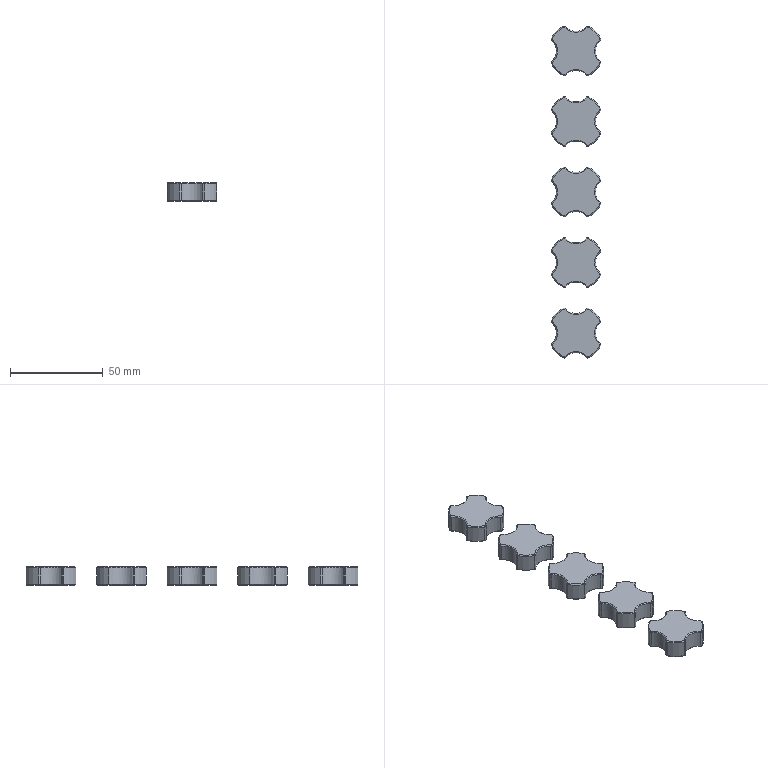NC program | NX | posted with a generic post | part box 26.875 x 178.875 x 10 mm
Whole program:
N10 G17 G21 G94 G90
(FLOOR_WALL_COPY , TOOL : D80)
N12 T19 M6
N14 G54
N16 G17 G0 G90 X-134.438 Y0. S6500 M3
N18 G43 Z30. H19
N20 Z7.5
N22 G94 G1 Z4.5 F1500.
N24 X-129.438
N26 X129.437
N28 X134.437
N30 Z7.5
N32 G0 Z30.
N34 X-134.438
N36 Z7.
N38 G1 Z4.
N40 X-129.438
N42 X129.437
N44 X134.437
N46 Z7.
N48 G0 Z30.
N50 X-134.438
N52 Z6.5
N54 G1 Z3.5
N56 X-129.438
N58 X129.437
N60 X134.437
N62 Z6.5
N64 G0 Z30.
N66 X-134.438
N68 Z6.
N70 G1 Z3.
N72 X-129.438
N74 X129.437
N76 X134.437
N78 Z6.
N80 G0 Z30.
N82 X-134.438
N84 Z5.5
N86 G1 Z2.5
N88 X-129.438
N90 X129.437
N92 X134.437
N94 Z5.5
N96 G0 Z30.
N98 X-134.438
N100 Z5.
N102 G1 Z2.
N104 X-129.438
N106 X129.437
N108 X134.437
N110 Z5.
N112 G0 Z30.
N114 X-134.438
N116 Z4.5
N118 G1 Z1.5
N120 X-129.438
N122 X129.437
N124 X134.437
N126 Z4.5
N128 G0 Z30.
N130 X-134.438
N132 Z4.
N134 G1 Z1.
N136 X-129.438
N138 X129.437
N140 X134.437
N142 Z4.
N144 G0 Z30.
N146 X-134.438
N148 Z3.5
N150 G1 Z0.5
N152 X-129.438
N154 X129.437
N156 X134.437
N158 Z3.5
N160 G0 Z30.
N162 X-134.438
N164 Z3.
N166 G1 Z0.
N168 X-129.438
N170 X129.437
N172 X134.437
N174 Z3.
N176 G0 Z30.
N178 M5
(PLANAR_MILL_COPY_COPY_COPY_COPY_COPY , TOOL : D6A45)
N180 T01 M6
N182 G54
N184 G17 G0 G90 X-64.945 Y12.28 S9500 M3
N186 G43 Z30. H1
N188 Z0.
N190 G94 G1 Z-1.5 F1250.
N192 G3 X-64.686 Y11.314 R1.
N194 G2 X-61.786 Y7.345 R16.
N196 X-62.254 Y4.915 R2.
N198 G3 X-62.254 Y-4.915 R6.5
N200 G2 X-61.786 Y-7.345 R2.
N202 X-68.655 Y-14.214 R16.
N204 X-71.085 Y-13.746 R2.
N206 G3 X-80.915 Y-13.746 R6.5
N208 G2 X-83.345 Y-14.214 R2.
N210 X-90.214 Y-7.345 R16.
N212 X-89.746 Y-4.915 R2.
N214 G3 X-89.746 Y4.915 R6.5
N216 G2 X-90.214 Y7.345 R2.
N218 X-83.345 Y14.214 R16.
N220 X-80.915 Y13.746 R2.
N222 G3 X-71.085 Y13.746 R6.5
N224 G2 X-68.655 Y14.214 R2.
N226 X-64.686 Y11.314 R16.
N228 G3 X-63.72 Y11.055 R1.
N230 G1 Z0.
N232 G0 Z30.
N234 X-50.28
N236 Z0.
N238 G1 Z-1.5
N240 G3 X-49.314 Y11.314 R1.
N242 G2 X-45.345 Y14.214 R16.
N244 X-42.915 Y13.746 R2.
N246 G3 X-33.085 Y13.746 R6.5
N248 G2 X-30.655 Y14.214 R2.
N250 X-23.786 Y7.345 R16.
N252 X-24.254 Y4.915 R2.
N254 G3 X-24.254 Y-4.915 R6.5
N256 G2 X-23.786 Y-7.345 R2.
N258 X-30.655 Y-14.214 R16.
N260 X-33.085 Y-13.746 R2.
N262 G3 X-42.915 Y-13.746 R6.5
N264 G2 X-45.345 Y-14.214 R2.
N266 X-52.214 Y-7.345 R16.
N268 X-51.746 Y-4.915 R2.
N270 G3 X-51.746 Y4.915 R6.5
N272 G2 X-52.214 Y7.345 R2.
N274 X-49.314 Y11.314 R16.
N276 G3 X-49.055 Y12.28 R1.
N278 G1 Z0.
N280 G0 Z30.
N282 X-12.28 Y11.055
N284 Z0.
N286 G1 Z-1.5
N288 G3 X-11.314 Y11.314 R1.
N290 G2 X-7.345 Y14.214 R16.
N292 X-4.915 Y13.746 R2.
N294 G3 X4.915 Y13.746 R6.5
N296 G2 X7.345 Y14.214 R2.
N298 X14.214 Y7.345 R16.
N300 X13.746 Y4.915 R2.
N302 G3 X13.746 Y-4.915 R6.5
N304 G2 X14.214 Y-7.345 R2.
N306 X7.345 Y-14.214 R16.
N308 X4.915 Y-13.746 R2.
N310 G3 X-4.915 Y-13.746 R6.5
N312 G2 X-7.345 Y-14.214 R2.
N314 X-14.214 Y-7.345 R16.
N316 X-13.746 Y-4.915 R2.
N318 G3 X-13.746 Y4.915 R6.5
N320 G2 X-14.214 Y7.345 R2.
N322 X-11.314 Y11.314 R16.
N324 G3 X-11.055 Y12.28 R1.
N326 G1 Z0.
N328 G0 Z30.
N330 X25.72 Y11.055
N332 Z0.
N334 G1 Z-1.5
N336 G3 X26.686 Y11.314 R1.
N338 G2 X30.655 Y14.214 R16.
N340 X33.085 Y13.746 R2.
N342 G3 X42.915 Y13.746 R6.5
N344 G2 X45.345 Y14.214 R2.
N346 X52.214 Y7.345 R16.
N348 X51.746 Y4.915 R2.
N350 G3 X51.746 Y-4.915 R6.5
N352 G2 X52.214 Y-7.345 R2.
N354 X45.345 Y-14.214 R16.
N356 X42.915 Y-13.746 R2.
N358 G3 X33.085 Y-13.746 R6.5
N360 G2 X30.655 Y-14.214 R2.
N362 X23.786 Y-7.345 R16.
N364 X24.254 Y-4.915 R2.
N366 G3 X24.254 Y4.915 R6.5
N368 G2 X23.786 Y7.345 R2.
N370 X26.686 Y11.314 R16.
N372 G3 X26.945 Y12.28 R1.
N374 G1 Z0.
N376 G0 Z30.
N378 X63.72 Y11.055
N380 Z0.
N382 G1 Z-1.5
N384 G3 X64.686 Y11.314 R1.
N386 G2 X68.655 Y14.214 R16.
N388 X71.085 Y13.746 R2.
N390 G3 X80.915 Y13.746 R6.5
N392 G2 X83.345 Y14.214 R2.
N394 X90.214 Y7.345 R16.
N396 X89.746 Y4.915 R2.
N398 G3 X89.746 Y-4.915 R6.5
N400 G2 X90.214 Y-7.345 R2.
N402 X83.345 Y-14.214 R16.
N404 X80.915 Y-13.746 R2.
N406 G3 X71.085 Y-13.746 R6.5
N408 G2 X68.655 Y-14.214 R2.
N410 X61.786 Y-7.345 R16.
N412 X62.254 Y-4.915 R2.
N414 G3 X62.254 Y4.915 R6.5
N416 G2 X61.786 Y7.345 R2.
N418 X64.686 Y11.314 R16.
N420 G3 X64.945 Y12.28 R1.
N422 G1 Z0.
N424 G0 Z30.
N426 M5
N428 M2